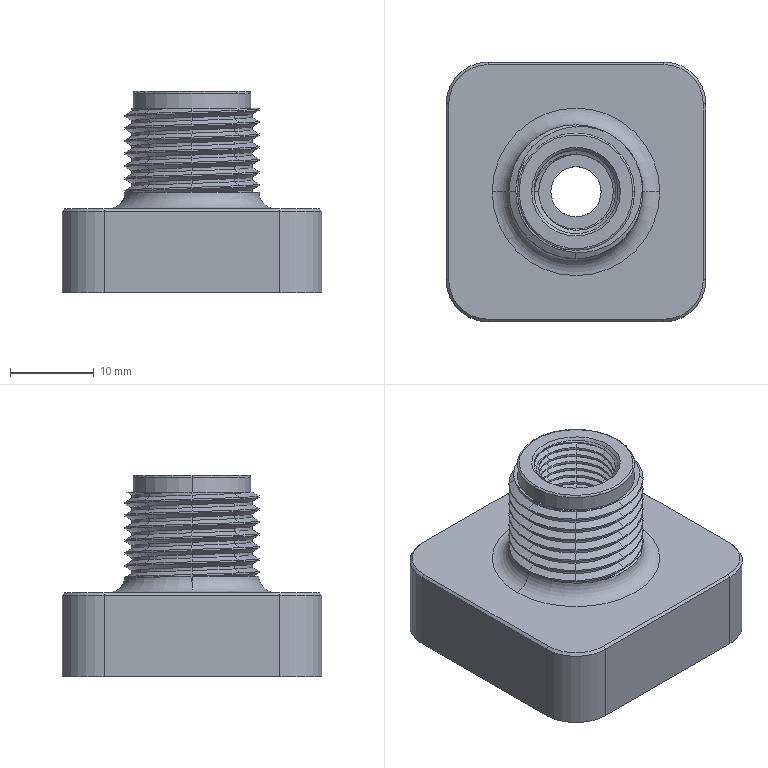Part | NX | features BREP 1 | 1 solid | 1343 faces | box 31 x 31 x 24 mm | volume 8742 mm3 | spline 786 | cylinder 507 | plane 28 | cone 18 | torus 4 | commonest cylinder face diameters 3.242 x212 4 x80 14.376 x66 8.917 x53 11.376 x33 16 x19